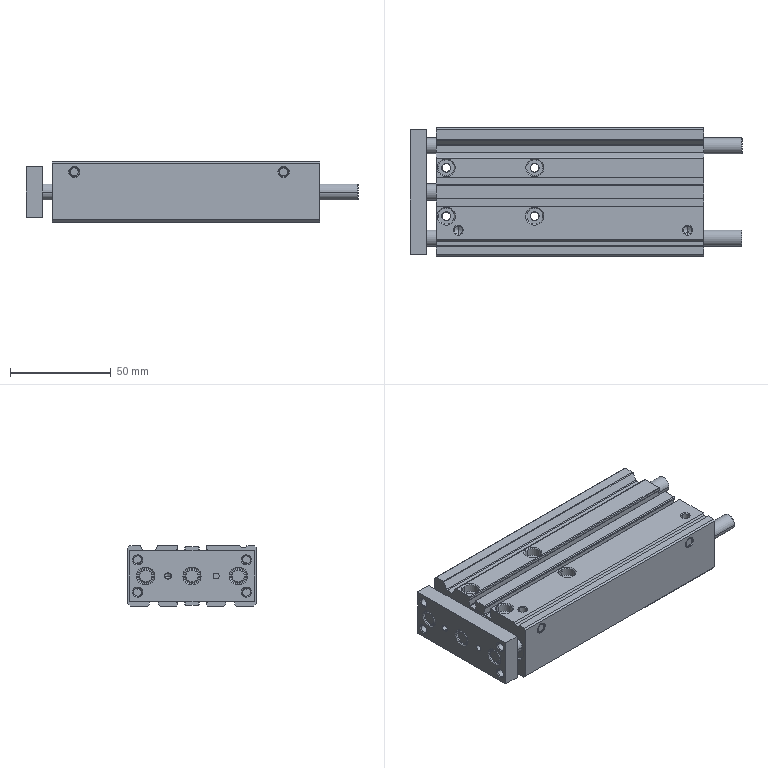Part | SolidWorks | features BaseBody 2 | 2 solids | 387 faces | box 165 x 64 x 30 mm | volume 211731 mm3 | cylinder 165 | plane 122 | cone 98 | spline 2 | commonest cylinder face diameters 4.134 x28 8 x26 3 x21 0.8 x20 0.4 x16 4.5 x8